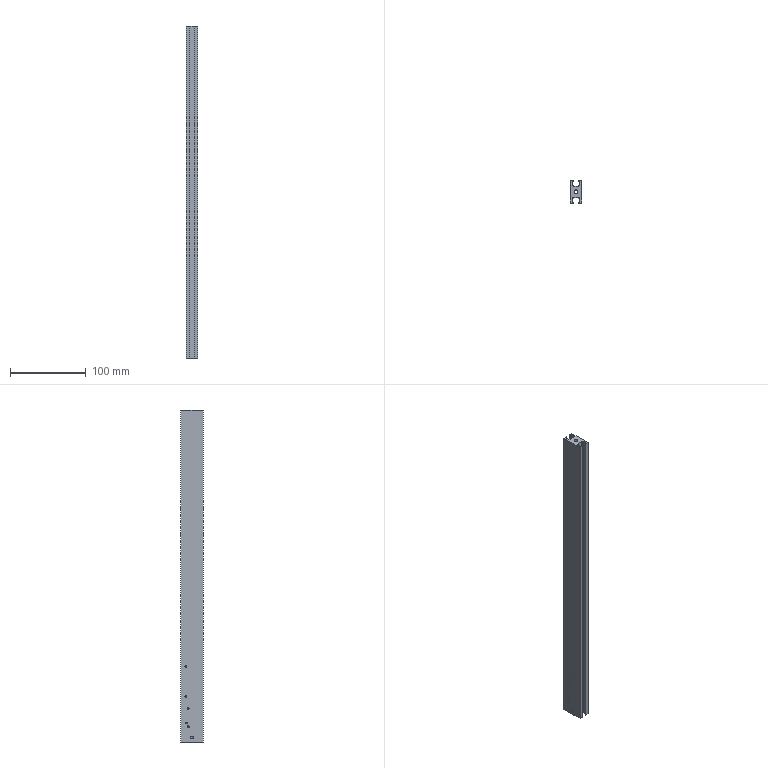Part | SolidWorks | features BaseBody 1 | 1 solid | 61 faces | box 15 x 30 x 438 mm | volume 123101 mm3 | plane 36 | cylinder 16 | cone 9 | commonest cylinder face diameters 2.5 x10 3.3 x4 5 x2